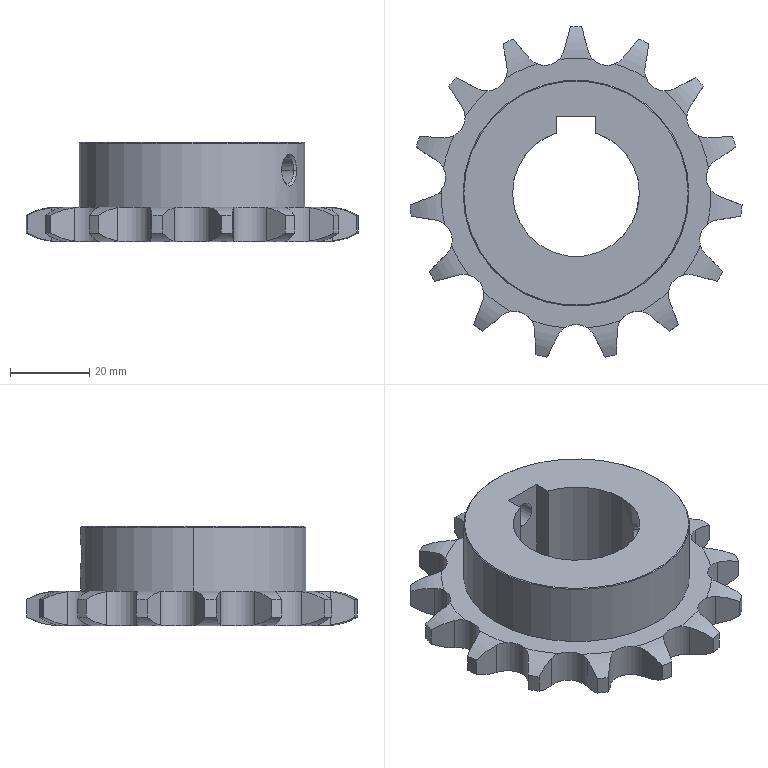Part | STEP file | _BSP50B15-N-32_B.stp | 1 solid | 118 faces | box 83.791 x 83.357 x 25 mm | volume 55752 mm3 | cylinder 44 | plane 36 | torus 32 | cone 6 | commonest cylinder face diameters 10.16 x20 84 x15 6.647 x4 32 x3 57 x2